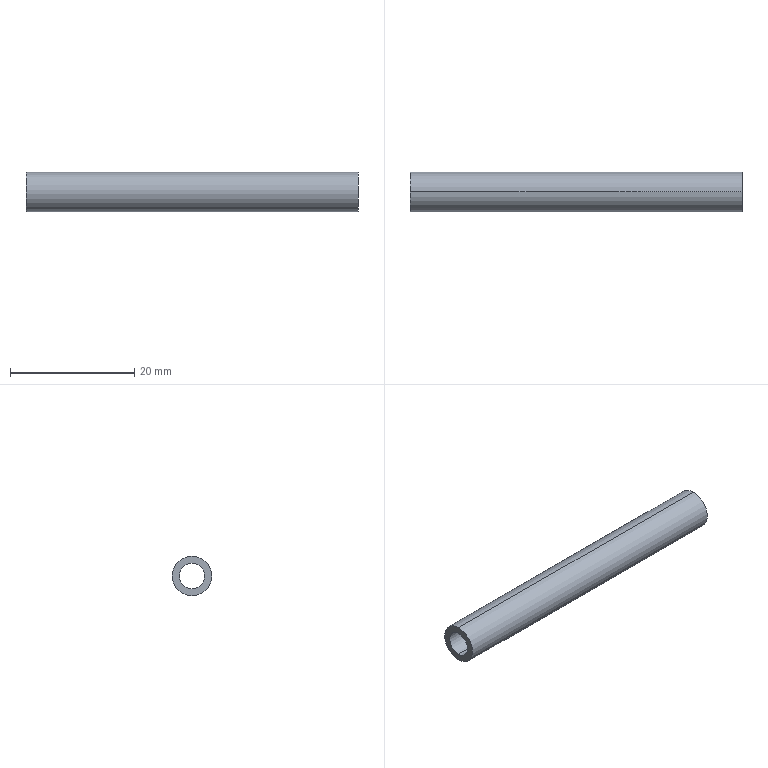Part | STEP file | GRM4_B10_TUBE_M_71195-001-002100 | 1 solid | 6 faces | box 53.34 x 6.35 x 6.35 mm | volume 997.325 mm3 | cylinder 4 | plane 2 | commonest cylinder face diameters 4.064 x2 6.35 x2
STEP:
#1=CARTESIAN_POINT('',(0.,0.,-3.175));
#2=VERTEX_POINT('',#1);
#3=CARTESIAN_POINT('',(0.,0.,3.175));
#4=VERTEX_POINT('',#3);
#5=CARTESIAN_POINT('',(0.,0.,0.));
#6=DIRECTION('',(1.,0.,0.));
#7=DIRECTION('',(0.,0.,-1.));
#8=AXIS2_PLACEMENT_3D('',#5,#6,#7);
#9=CIRCLE('',#8,3.175);
#10=EDGE_CURVE('',#2,#4,#9,.T.);
#11=ORIENTED_EDGE('',*,*,#10,.T.);
#12=CARTESIAN_POINT('',(53.34,0.,3.175));
#13=VERTEX_POINT('',#12);
#14=CARTESIAN_POINT('',(53.34,0.,3.175));
#15=DIRECTION('',(1.,0.,0.));
#16=VECTOR('',#15,1000.);
#17=LINE('',#14,#16);
#18=EDGE_CURVE('',#4,#13,#17,.T.);
#19=ORIENTED_EDGE('',*,*,#18,.T.);
#20=CARTESIAN_POINT('',(53.34,0.,-3.175));
#21=VERTEX_POINT('',#20);
#22=CARTESIAN_POINT('',(53.34,0.,0.));
#23=DIRECTION('',(-1.,0.,0.));
#24=DIRECTION('',(0.,0.,-1.));
#25=AXIS2_PLACEMENT_3D('',#22,#23,#24);
#26=CIRCLE('',#25,3.175);
#27=EDGE_CURVE('',#13,#21,#26,.T.);
#28=ORIENTED_EDGE('',*,*,#27,.T.);
#29=CARTESIAN_POINT('',(53.34,0.,-3.175));
#30=DIRECTION('',(1.,0.,0.));
#31=VECTOR('',#30,1000.);
#32=LINE('',#29,#31);
#33=EDGE_CURVE('',#2,#21,#32,.T.);
#34=ORIENTED_EDGE('',*,*,#33,.F.);
#35=EDGE_LOOP('',(#11,#19,#28,#34));
#36=FACE_OUTER_BOUND('',#35,.T.);
#37=CARTESIAN_POINT('',(53.34,0.,0.));
#38=DIRECTION('',(1.,0.,0.));
#39=DIRECTION('',(0.,0.,-1.));
#40=AXIS2_PLACEMENT_3D('',#37,#38,#39);
#41=CYLINDRICAL_SURFACE('',#40,3.175);
#42=ADVANCED_FACE('',(#36),#41,.T.);
#43=CARTESIAN_POINT('',(0.,0.,2.032));
#44=VERTEX_POINT('',#43);
#45=CARTESIAN_POINT('',(0.,0.,-2.032));
#46=VERTEX_POINT('',#45);
#47=CARTESIAN_POINT('',(0.,0.,0.));
#48=DIRECTION('',(1.,0.,0.));
#49=DIRECTION('',(0.,0.,-1.));
#50=AXIS2_PLACEMENT_3D('',#47,#48,#49);
#51=CIRCLE('',#50,2.032);
#52=EDGE_CURVE('',#44,#46,#51,.T.);
#53=ORIENTED_EDGE('',*,*,#52,.F.);
#54=CARTESIAN_POINT('',(53.34,0.,2.032));
#55=VERTEX_POINT('',#54);
#56=CARTESIAN_POINT('',(53.34,0.,2.032));
#57=DIRECTION('',(1.,0.,0.));
#58=VECTOR('',#57,1000.);
#59=LINE('',#56,#58);
#60=EDGE_CURVE('',#44,#55,#59,.T.);
#61=ORIENTED_EDGE('',*,*,#60,.T.);
#62=CARTESIAN_POINT('',(53.34,0.,-2.032));
#63=VERTEX_POINT('',#62);
#64=CARTESIAN_POINT('',(53.34,0.,0.));
#65=DIRECTION('',(-1.,0.,0.));
#66=DIRECTION('',(0.,0.,-1.));
#67=AXIS2_PLACEMENT_3D('',#64,#65,#66);
#68=CIRCLE('',#67,2.032);
#69=EDGE_CURVE('',#63,#55,#68,.T.);
#70=ORIENTED_EDGE('',*,*,#69,.F.);
#71=CARTESIAN_POINT('',(53.34,0.,-2.032));
#72=DIRECTION('',(1.,0.,0.));
#73=VECTOR('',#72,1000.);
#74=LINE('',#71,#73);
#75=EDGE_CURVE('',#46,#63,#74,.T.);
#76=ORIENTED_EDGE('',*,*,#75,.F.);
#77=EDGE_LOOP('',(#53,#61,#70,#76));
#78=FACE_OUTER_BOUND('',#77,.T.);
#79=CARTESIAN_POINT('',(53.34,0.,0.));
#80=DIRECTION('',(1.,0.,0.));
#81=DIRECTION('',(0.,0.,-1.));
#82=AXIS2_PLACEMENT_3D('',#79,#80,#81);
#83=CYLINDRICAL_SURFACE('',#82,2.032);
#84=ADVANCED_FACE('',(#78),#83,.F.);
#85=ORIENTED_EDGE('',*,*,#18,.F.);
#86=CARTESIAN_POINT('',(0.,0.,0.));
#87=DIRECTION('',(1.,0.,0.));
#88=DIRECTION('',(0.,0.,-1.));
#89=AXIS2_PLACEMENT_3D('',#86,#87,#88);
#90=CIRCLE('',#89,3.175);
#91=EDGE_CURVE('',#4,#2,#90,.T.);
#92=ORIENTED_EDGE('',*,*,#91,.T.);
#93=ORIENTED_EDGE('',*,*,#33,.T.);
#94=CARTESIAN_POINT('',(53.34,0.,0.));
#95=DIRECTION('',(-1.,0.,0.));
#96=DIRECTION('',(0.,0.,-1.));
#97=AXIS2_PLACEMENT_3D('',#94,#95,#96);
#98=CIRCLE('',#97,3.175);
#99=EDGE_CURVE('',#21,#13,#98,.T.);
#100=ORIENTED_EDGE('',*,*,#99,.T.);
#101=EDGE_LOOP('',(#85,#92,#93,#100));
#102=FACE_OUTER_BOUND('',#101,.T.);
#103=CARTESIAN_POINT('',(53.34,0.,0.));
#104=DIRECTION('',(1.,0.,0.));
#105=DIRECTION('',(0.,0.,-1.));
#106=AXIS2_PLACEMENT_3D('',#103,#104,#105);
#107=CYLINDRICAL_SURFACE('',#106,3.175);
#108=ADVANCED_FACE('',(#102),#107,.T.);
#109=ORIENTED_EDGE('',*,*,#69,.T.);
#110=CARTESIAN_POINT('',(53.34,0.,0.));
#111=DIRECTION('',(-1.,0.,0.));
#112=DIRECTION('',(0.,0.,-1.));
#113=AXIS2_PLACEMENT_3D('',#110,#111,#112);
#114=CIRCLE('',#113,2.032);
#115=EDGE_CURVE('',#55,#63,#114,.T.);
#116=ORIENTED_EDGE('',*,*,#115,.T.);
#117=EDGE_LOOP('',(#109,#116));
#118=FACE_BOUND('',#117,.T.);
#119=ORIENTED_EDGE('',*,*,#99,.F.);
#120=ORIENTED_EDGE('',*,*,#27,.F.);
#121=EDGE_LOOP('',(#119,#120));
#122=FACE_OUTER_BOUND('',#121,.T.);
#123=CARTESIAN_POINT('',(53.34,2.032,0.));
#124=DIRECTION('',(1.,0.,0.));
#125=DIRECTION('',(0.,0.,-1.));
#126=AXIS2_PLACEMENT_3D('',#123,#124,#125);
#127=PLANE('',#126);
#128=ADVANCED_FACE('',(#118,#122),#127,.T.);
#129=ORIENTED_EDGE('',*,*,#10,.F.);
#130=ORIENTED_EDGE('',*,*,#91,.F.);
#131=EDGE_LOOP('',(#129,#130));
#132=FACE_OUTER_BOUND('',#131,.T.);
#133=CARTESIAN_POINT('',(0.,0.,0.));
#134=DIRECTION('',(1.,0.,0.));
#135=DIRECTION('',(0.,0.,-1.));
#136=AXIS2_PLACEMENT_3D('',#133,#134,#135);
#137=CIRCLE('',#136,2.032);
#138=EDGE_CURVE('',#46,#44,#137,.T.);
#139=ORIENTED_EDGE('',*,*,#138,.T.);
#140=ORIENTED_EDGE('',*,*,#52,.T.);
#141=EDGE_LOOP('',(#139,#140));
#142=FACE_BOUND('',#141,.T.);
#143=CARTESIAN_POINT('',(0.,3.175,0.));
#144=DIRECTION('',(-1.,0.,0.));
#145=DIRECTION('',(0.,0.,1.));
#146=AXIS2_PLACEMENT_3D('',#143,#144,#145);
#147=PLANE('',#146);
#148=ADVANCED_FACE('',(#132,#142),#147,.T.);
#149=ORIENTED_EDGE('',*,*,#60,.F.);
#150=ORIENTED_EDGE('',*,*,#138,.F.);
#151=ORIENTED_EDGE('',*,*,#75,.T.);
#152=ORIENTED_EDGE('',*,*,#115,.F.);
#153=EDGE_LOOP('',(#149,#150,#151,#152));
#154=FACE_OUTER_BOUND('',#153,.T.);
#155=CARTESIAN_POINT('',(53.34,0.,0.));
#156=DIRECTION('',(1.,0.,0.));
#157=DIRECTION('',(0.,0.,-1.));
#158=AXIS2_PLACEMENT_3D('',#155,#156,#157);
#159=CYLINDRICAL_SURFACE('',#158,2.032);
#160=ADVANCED_FACE('',(#154),#159,.F.);
#161=CLOSED_SHELL('',(#42,#84,#108,#128,#148,#160));
#162=MANIFOLD_SOLID_BREP('',#161);
#163=CARTESIAN_POINT('',(0.,0.,0.));
#164=DIRECTION('',(0.,0.,1.));
#165=DIRECTION('',(1.,0.,0.));
#166=AXIS2_PLACEMENT_3D('',#163,#164,#165);
#167=(LENGTH_UNIT()NAMED_UNIT(*)SI_UNIT(.MILLI.,.METRE.));
#168=UNCERTAINTY_MEASURE_WITH_UNIT(LENGTH_MEASURE(0.00001),#167,'','');
#169=(NAMED_UNIT(*)PLANE_ANGLE_UNIT()SI_UNIT($,.RADIAN.));
#170=(NAMED_UNIT(*)SI_UNIT($,.STERADIAN.)SOLID_ANGLE_UNIT());
#171=(GEOMETRIC_REPRESENTATION_CONTEXT(3)GLOBAL_UNCERTAINTY_ASSIGNED_CONTEXT((#168))GLOBAL_UNIT_ASSIGNED_CONTEXT((#167,#169,#170))REPRESENTATION_CONTEXT('',''));
#172=ADVANCED_BREP_SHAPE_REPRESENTATION('',(#162,#166),#171);